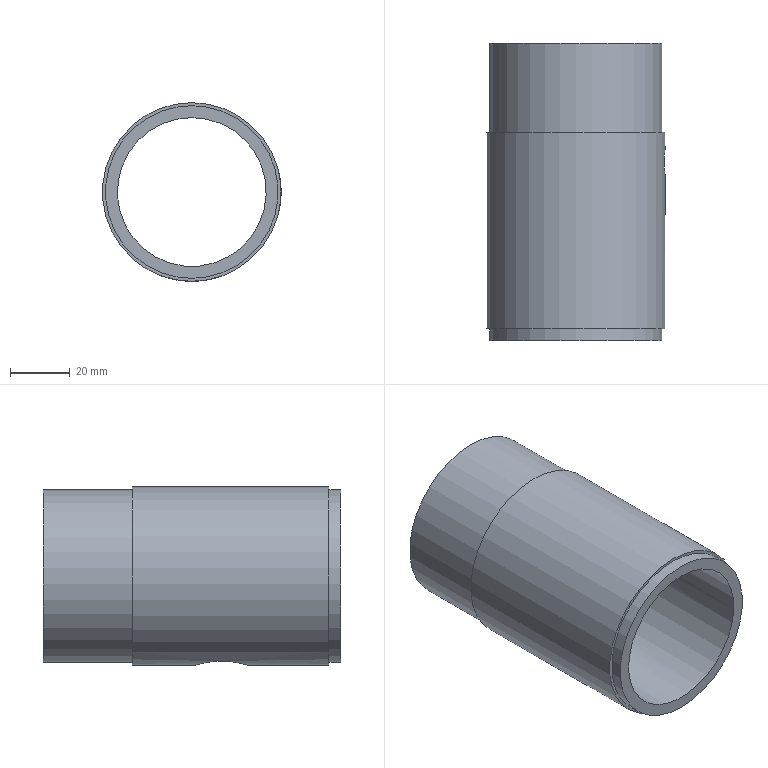Part | STEP file | JBJ-P-1008-02 | 1 solid | 10 faces | box 60 x 100 x 60 mm | volume 77175 mm3 | cylinder 6 | plane 3 | cone 1 | commonest cylinder face diameters 58 x2 8.8 x1 18 x1 50 x1 60 x1
STEP:
#1=CARTESIAN_POINT('',(0.,49.,-30.));
#2=VERTEX_POINT('',#1);
#3=CARTESIAN_POINT('',(0.,49.,-30.));
#4=CARTESIAN_POINT('',(-0.5983,49.,-30.));
#5=CARTESIAN_POINT('',(-1.186,48.941,-29.982));
#6=CARTESIAN_POINT('',(-2.052,48.768,-29.931));
#7=CARTESIAN_POINT('',(-2.338,48.696,-29.91));
#8=CARTESIAN_POINT('',(-2.906,48.523,-29.86));
#9=CARTESIAN_POINT('',(-3.187,48.422,-29.832));
#10=CARTESIAN_POINT('',(-4.003,48.082,-29.737));
#11=CARTESIAN_POINT('',(-4.518,47.806,-29.662));
#12=CARTESIAN_POINT('',(-5.25,47.316,-29.538));
#13=CARTESIAN_POINT('',(-5.488,47.139,-29.495));
#14=CARTESIAN_POINT('',(-5.943,46.765,-29.406));
#15=CARTESIAN_POINT('',(-6.16,46.569,-29.362));
#16=CARTESIAN_POINT('',(-6.778,45.95,-29.227));
#17=CARTESIAN_POINT('',(-7.149,45.499,-29.138));
#18=CARTESIAN_POINT('',(-7.807,44.516,-28.968));
#19=CARTESIAN_POINT('',(-8.084,43.998,-28.891));
#20=CARTESIAN_POINT('',(-8.422,43.187,-28.794));
#21=CARTESIAN_POINT('',(-8.521,42.911,-28.764));
#22=CARTESIAN_POINT('',(-8.694,42.346,-28.713));
#23=CARTESIAN_POINT('',(-8.767,42.056,-28.69));
#24=CARTESIAN_POINT('',(-8.942,41.183,-28.637));
#25=CARTESIAN_POINT('',(-9.,40.597,-28.618));
#26=CARTESIAN_POINT('',(-9.,39.415,-28.618));
#27=CARTESIAN_POINT('',(-8.941,38.815,-28.637));
#28=CARTESIAN_POINT('',(-8.71,37.658,-28.708));
#29=CARTESIAN_POINT('',(-8.539,37.095,-28.76));
#30=CARTESIAN_POINT('',(-8.198,36.275,-28.858));
#31=CARTESIAN_POINT('',(-8.071,36.006,-28.894));
#32=CARTESIAN_POINT('',(-7.793,35.488,-28.971));
#33=CARTESIAN_POINT('',(-7.642,35.238,-29.011));
#34=CARTESIAN_POINT('',(-7.317,34.752,-29.094));
#35=CARTESIAN_POINT('',(-7.143,34.517,-29.138));
#36=CARTESIAN_POINT('',(-6.771,34.063,-29.227));
#37=CARTESIAN_POINT('',(-6.572,33.844,-29.272));
#38=CARTESIAN_POINT('',(-5.949,33.221,-29.407));
#39=CARTESIAN_POINT('',(-5.498,32.851,-29.496));
#40=CARTESIAN_POINT('',(-4.526,32.199,-29.661));
#41=CARTESIAN_POINT('',(-3.999,31.916,-29.737));
#42=CARTESIAN_POINT('',(-2.914,31.465,-29.863));
#43=CARTESIAN_POINT('',(-2.353,31.293,-29.913));
#44=CARTESIAN_POINT('',(-1.481,31.118,-29.965));
#45=CARTESIAN_POINT('',(-1.184,31.073,-29.978));
#46=CARTESIAN_POINT('',(-0.5936,31.015,-29.996));
#47=CARTESIAN_POINT('',(-0.003551,30.986,-30.004));
#48=CARTESIAN_POINT('',(0.5855,31.014,-29.996));
#49=CARTESIAN_POINT('',(1.174,31.072,-29.978));
#50=CARTESIAN_POINT('',(1.469,31.116,-29.965));
#51=CARTESIAN_POINT('',(2.346,31.291,-29.914));
#52=CARTESIAN_POINT('',(2.909,31.463,-29.864));
#53=CARTESIAN_POINT('',(3.994,31.913,-29.738));
#54=CARTESIAN_POINT('',(4.521,32.196,-29.662));
#55=CARTESIAN_POINT('',(5.495,32.848,-29.497));
#56=CARTESIAN_POINT('',(5.946,33.218,-29.408));
#57=CARTESIAN_POINT('',(6.569,33.841,-29.273));
#58=CARTESIAN_POINT('',(6.768,34.061,-29.227));
#59=CARTESIAN_POINT('',(7.141,34.514,-29.138));
#60=CARTESIAN_POINT('',(7.315,34.749,-29.095));
#61=CARTESIAN_POINT('',(7.802,35.476,-28.97));
#62=CARTESIAN_POINT('',(8.081,35.993,-28.892));
#63=CARTESIAN_POINT('',(8.537,37.09,-28.761));
#64=CARTESIAN_POINT('',(8.708,37.653,-28.709));
#65=CARTESIAN_POINT('',(8.882,38.518,-28.655));
#66=CARTESIAN_POINT('',(8.926,38.81,-28.641));
#67=CARTESIAN_POINT('',(8.985,39.401,-28.623));
#68=CARTESIAN_POINT('',(9.,39.701,-28.618));
#69=CARTESIAN_POINT('',(9.,40.591,-28.618));
#70=CARTESIAN_POINT('',(8.942,41.177,-28.637));
#71=CARTESIAN_POINT('',(8.769,42.047,-28.69));
#72=CARTESIAN_POINT('',(8.696,42.337,-28.712));
#73=CARTESIAN_POINT('',(8.524,42.905,-28.764));
#74=CARTESIAN_POINT('',(8.424,43.182,-28.793));
#75=CARTESIAN_POINT('',(8.086,43.995,-28.891));
#76=CARTESIAN_POINT('',(7.809,44.513,-28.968));
#77=CARTESIAN_POINT('',(7.151,45.497,-29.137));
#78=CARTESIAN_POINT('',(6.78,45.948,-29.227));
#79=CARTESIAN_POINT('',(6.161,46.567,-29.361));
#80=CARTESIAN_POINT('',(5.944,46.764,-29.406));
#81=CARTESIAN_POINT('',(5.49,47.137,-29.494));
#82=CARTESIAN_POINT('',(5.252,47.315,-29.538));
#83=CARTESIAN_POINT('',(4.52,47.805,-29.662));
#84=CARTESIAN_POINT('',(4.005,48.081,-29.736));
#85=CARTESIAN_POINT('',(2.919,48.534,-29.863));
#86=CARTESIAN_POINT('',(2.345,48.709,-29.914));
#87=CARTESIAN_POINT('',(1.187,48.941,-29.982));
#88=CARTESIAN_POINT('',(0.5983,49.,-30.));
#89=CARTESIAN_POINT('',(0.,49.,-30.));
#90=B_SPLINE_CURVE_WITH_KNOTS('',3,(#3,#4,#5,#6,#7,#8,#9,#10,#11,#12,#13,#14,#15,#16,#17,#18,#19,#20,#21,#22,#23,#24,#25,#26,#27,#28,#29,#30,#31,#32,#33,#34,#35,#36,#37,#38,#39,#40,#41,#42,#43,#44,#45,#46,#47,#48,#49,#50,#51,#52,#53,#54,#55,#56,#57,#58,#59,#60,#61,#62,#63,#64,#65,#66,#67,#68,#69,#70,#71,#72,#73,#74,#75,#76,#77,#78,#79,#80,#81,#82,#83,#84,#85,#86,#87,#88,#89),.UNSPECIFIED.,.T.,.F.,(4,2,2,2,2,2,2,2,2,2,2,2,2,2,2,2,2,2,2,2,2,2,1,2,2,2,2,2,2,2,2,2,2,2,2,2,2,2,2,2,2,2,2,4),(0.,0.001769,0.002653,0.003537,0.005306,0.00619,0.007075,0.008843,0.01061,0.0115,0.01238,0.01415,0.01592,0.01769,0.01857,0.01946,0.02034,0.02122,0.02299,0.02476,0.02653,0.02741,0.0283,0.02918,0.03007,0.03184,0.0336,0.03537,0.03626,0.03714,0.03891,0.04068,0.04156,0.04245,0.04422,0.0451,0.04598,0.04775,0.04952,0.05041,0.05129,0.05306,0.05483,0.0566),.UNSPECIFIED.);
#91=EDGE_CURVE('',#2,#2,#90,.T.);
#92=ORIENTED_EDGE('',*,*,#91,.T.);
#93=EDGE_LOOP('',(#92));
#94=FACE_BOUND('',#93,.T.);
#95=CARTESIAN_POINT('',(30.,55.6,0.));
#96=VERTEX_POINT('',#95);
#97=CARTESIAN_POINT('',(30.,55.6,0.));
#98=CARTESIAN_POINT('',(30.,55.6,0.2911));
#99=CARTESIAN_POINT('',(29.996,55.629,0.5773));
#100=CARTESIAN_POINT('',(29.98,55.741,1.14));
#101=CARTESIAN_POINT('',(29.968,55.825,1.42));
#102=CARTESIAN_POINT('',(29.938,56.046,1.952));
#103=CARTESIAN_POINT('',(29.92,56.182,2.205));
#104=CARTESIAN_POINT('',(29.881,56.501,2.683));
#105=CARTESIAN_POINT('',(29.859,56.686,2.909));
#106=CARTESIAN_POINT('',(29.817,57.092,3.314));
#107=CARTESIAN_POINT('',(29.796,57.313,3.496));
#108=CARTESIAN_POINT('',(29.757,57.794,3.818));
#109=CARTESIAN_POINT('',(29.738,58.049,3.954));
#110=CARTESIAN_POINT('',(29.708,58.579,4.174));
#111=CARTESIAN_POINT('',(29.696,58.856,4.259));
#112=CARTESIAN_POINT('',(29.68,59.424,4.372));
#113=CARTESIAN_POINT('',(29.676,59.71,4.4));
#114=CARTESIAN_POINT('',(29.676,60.285,4.4));
#115=CARTESIAN_POINT('',(29.68,60.577,4.372));
#116=CARTESIAN_POINT('',(29.696,61.141,4.259));
#117=CARTESIAN_POINT('',(29.708,61.416,4.176));
#118=CARTESIAN_POINT('',(29.738,61.949,3.955));
#119=CARTESIAN_POINT('',(29.757,62.206,3.818));
#120=CARTESIAN_POINT('',(29.796,62.683,3.499));
#121=CARTESIAN_POINT('',(29.817,62.905,3.317));
#122=CARTESIAN_POINT('',(29.859,63.315,2.907));
#123=CARTESIAN_POINT('',(29.881,63.497,2.686));
#124=CARTESIAN_POINT('',(29.919,63.816,2.21));
#125=CARTESIAN_POINT('',(29.938,63.954,1.952));
#126=CARTESIAN_POINT('',(29.968,64.175,1.42));
#127=CARTESIAN_POINT('',(29.979,64.258,1.145));
#128=CARTESIAN_POINT('',(29.996,64.371,0.5809));
#129=CARTESIAN_POINT('',(30.,64.4,0.289));
#130=CARTESIAN_POINT('',(30.,64.4,-0.2857));
#131=CARTESIAN_POINT('',(29.996,64.372,-0.5715));
#132=CARTESIAN_POINT('',(29.98,64.26,-1.14));
#133=CARTESIAN_POINT('',(29.968,64.175,-1.418));
#134=CARTESIAN_POINT('',(29.938,63.956,-1.947));
#135=CARTESIAN_POINT('',(29.92,63.819,-2.204));
#136=CARTESIAN_POINT('',(29.881,63.499,-2.684));
#137=CARTESIAN_POINT('',(29.86,63.317,-2.905));
#138=CARTESIAN_POINT('',(29.817,62.912,-3.311));
#139=CARTESIAN_POINT('',(29.796,62.686,-3.497));
#140=CARTESIAN_POINT('',(29.757,62.208,-3.816));
#141=CARTESIAN_POINT('',(29.739,61.956,-3.952));
#142=CARTESIAN_POINT('',(29.708,61.423,-4.173));
#143=CARTESIAN_POINT('',(29.696,61.144,-4.258));
#144=CARTESIAN_POINT('',(29.68,60.581,-4.371));
#145=CARTESIAN_POINT('',(29.676,60.295,-4.4));
#146=CARTESIAN_POINT('',(29.676,59.713,-4.4));
#147=CARTESIAN_POINT('',(29.68,59.427,-4.372));
#148=CARTESIAN_POINT('',(29.696,58.864,-4.26));
#149=CARTESIAN_POINT('',(29.708,58.584,-4.176));
#150=CARTESIAN_POINT('',(29.738,58.051,-3.955));
#151=CARTESIAN_POINT('',(29.756,57.798,-3.82));
#152=CARTESIAN_POINT('',(29.795,57.32,-3.501));
#153=CARTESIAN_POINT('',(29.817,57.094,-3.316));
#154=CARTESIAN_POINT('',(29.859,56.688,-2.911));
#155=CARTESIAN_POINT('',(29.88,56.506,-2.69));
#156=CARTESIAN_POINT('',(29.92,56.184,-2.209));
#157=CARTESIAN_POINT('',(29.937,56.047,-1.954));
#158=CARTESIAN_POINT('',(29.967,55.827,-1.425));
#159=CARTESIAN_POINT('',(29.979,55.742,-1.147));
#160=CARTESIAN_POINT('',(29.996,55.629,-0.5788));
#161=CARTESIAN_POINT('',(30.,55.6,-0.2911));
#162=CARTESIAN_POINT('',(30.,55.6,0.));
#163=B_SPLINE_CURVE_WITH_KNOTS('',3,(#97,#98,#99,#100,#101,#102,#103,#104,#105,#106,#107,#108,#109,#110,#111,#112,#113,#114,#115,#116,#117,#118,#119,#120,#121,#122,#123,#124,#125,#126,#127,#128,#129,#130,#131,#132,#133,#134,#135,#136,#137,#138,#139,#140,#141,#142,#143,#144,#145,#146,#147,#148,#149,#150,#151,#152,#153,#154,#155,#156,#157,#158,#159,#160,#161,#162),.UNSPECIFIED.,.T.,.F.,(4,2,2,2,2,2,2,2,2,2,2,2,2,2,2,2,2,2,2,2,2,2,2,2,2,2,2,2,2,2,2,2,4),(0.,0.0008608,0.001722,0.002582,0.003443,0.004304,0.005165,0.006026,0.006887,0.007747,0.008608,0.009469,0.01033,0.01119,0.01205,0.01291,0.01377,0.01463,0.01549,0.01636,0.01722,0.01808,0.01894,0.0198,0.02066,0.02152,0.02238,0.02324,0.0241,0.02496,0.02582,0.02669,0.02755),.UNSPECIFIED.);
#164=EDGE_CURVE('',#96,#96,#163,.T.);
#165=ORIENTED_EDGE('',*,*,#164,.T.);
#166=EDGE_LOOP('',(#165));
#167=FACE_BOUND('',#166,.T.);
#168=CARTESIAN_POINT('',(0.,4.,-30.));
#169=VERTEX_POINT('',#168);
#170=CARTESIAN_POINT('',(0.,4.,0.));
#171=DIRECTION('',(0.,-1.,0.));
#172=DIRECTION('',(0.,0.,-1.));
#173=AXIS2_PLACEMENT_3D('',#170,#171,#172);
#174=CIRCLE('',#173,30.);
#175=EDGE_CURVE('',#169,#169,#174,.T.);
#176=ORIENTED_EDGE('',*,*,#175,.F.);
#177=EDGE_LOOP('',(#176));
#178=FACE_OUTER_BOUND('',#177,.T.);
#179=CARTESIAN_POINT('',(0.,70.,30.));
#180=VERTEX_POINT('',#179);
#181=CARTESIAN_POINT('',(0.,70.,0.));
#182=DIRECTION('',(0.,1.,0.));
#183=DIRECTION('',(0.,0.,1.));
#184=AXIS2_PLACEMENT_3D('',#181,#182,#183);
#185=CIRCLE('',#184,30.);
#186=EDGE_CURVE('',#180,#180,#185,.T.);
#187=ORIENTED_EDGE('',*,*,#186,.F.);
#188=EDGE_LOOP('',(#187));
#189=FACE_OUTER_BOUND('',#188,.T.);
#190=CARTESIAN_POINT('',(0.,100.,0.));
#191=DIRECTION('',(0.,-1.,0.));
#192=DIRECTION('',(0.,0.,-1.));
#193=AXIS2_PLACEMENT_3D('',#190,#191,#192);
#194=CYLINDRICAL_SURFACE('',#193,30.);
#195=ADVANCED_FACE('',(#94,#167,#178,#189),#194,.T.);
#196=CARTESIAN_POINT('',(0.,0.,25.));
#197=VERTEX_POINT('',#196);
#198=CARTESIAN_POINT('',(0.,0.,0.));
#199=DIRECTION('',(0.,1.,0.));
#200=DIRECTION('',(0.,0.,1.));
#201=AXIS2_PLACEMENT_3D('',#198,#199,#200);
#202=CIRCLE('',#201,25.);
#203=EDGE_CURVE('',#197,#197,#202,.T.);
#204=ORIENTED_EDGE('',*,*,#203,.T.);
#205=EDGE_LOOP('',(#204));
#206=FACE_BOUND('',#205,.T.);
#207=CARTESIAN_POINT('',(0.,0.,-29.));
#208=VERTEX_POINT('',#207);
#209=CARTESIAN_POINT('',(0.,0.,0.));
#210=DIRECTION('',(0.,-1.,0.));
#211=DIRECTION('',(0.,0.,-1.));
#212=AXIS2_PLACEMENT_3D('',#209,#210,#211);
#213=CIRCLE('',#212,29.);
#214=EDGE_CURVE('',#208,#208,#213,.T.);
#215=ORIENTED_EDGE('',*,*,#214,.T.);
#216=EDGE_LOOP('',(#215));
#217=FACE_OUTER_BOUND('',#216,.T.);
#218=CARTESIAN_POINT('',(0.,0.,0.));
#219=DIRECTION('',(0.,1.,0.));
#220=DIRECTION('',(0.,0.,1.));
#221=AXIS2_PLACEMENT_3D('',#218,#219,#220);
#222=PLANE('',#221);
#223=ADVANCED_FACE('',(#206,#217),#222,.F.);
#224=CARTESIAN_POINT('',(0.,96.,25.));
#225=VERTEX_POINT('',#224);
#226=CARTESIAN_POINT('',(0.,96.,0.));
#227=DIRECTION('',(0.,1.,0.));
#228=DIRECTION('',(0.,0.,1.));
#229=AXIS2_PLACEMENT_3D('',#226,#227,#228);
#230=CIRCLE('',#229,25.);
#231=EDGE_CURVE('',#225,#225,#230,.T.);
#232=ORIENTED_EDGE('',*,*,#231,.T.);
#233=EDGE_LOOP('',(#232));
#234=FACE_OUTER_BOUND('',#233,.T.);
#235=CARTESIAN_POINT('',(0.,49.,-25.));
#236=VERTEX_POINT('',#235);
#237=CARTESIAN_POINT('',(0.,49.,-25.));
#238=CARTESIAN_POINT('',(-0.6,49.,-25.));
#239=CARTESIAN_POINT('',(-1.189,48.941,-24.978));
#240=CARTESIAN_POINT('',(-2.057,48.767,-24.917));
#241=CARTESIAN_POINT('',(-2.344,48.695,-24.892));
#242=CARTESIAN_POINT('',(-2.912,48.521,-24.831));
#243=CARTESIAN_POINT('',(-3.193,48.42,-24.797));
#244=CARTESIAN_POINT('',(-4.009,48.079,-24.683));
#245=CARTESIAN_POINT('',(-4.524,47.803,-24.592));
#246=CARTESIAN_POINT('',(-5.255,47.313,-24.443));
#247=CARTESIAN_POINT('',(-5.492,47.136,-24.39));
#248=CARTESIAN_POINT('',(-5.945,46.763,-24.284));
#249=CARTESIAN_POINT('',(-6.161,46.567,-24.23));
#250=CARTESIAN_POINT('',(-6.778,45.95,-24.067));
#251=CARTESIAN_POINT('',(-7.149,45.499,-23.959));
#252=CARTESIAN_POINT('',(-7.806,44.518,-23.753));
#253=CARTESIAN_POINT('',(-8.082,44.003,-23.659));
#254=CARTESIAN_POINT('',(-8.42,43.193,-23.54));
#255=CARTESIAN_POINT('',(-8.52,42.916,-23.504));
#256=CARTESIAN_POINT('',(-8.693,42.35,-23.44));
#257=CARTESIAN_POINT('',(-8.766,42.059,-23.413));
#258=CARTESIAN_POINT('',(-8.941,41.186,-23.347));
#259=CARTESIAN_POINT('',(-9.,40.599,-23.324));
#260=CARTESIAN_POINT('',(-9.,39.71,-23.324));
#261=CARTESIAN_POINT('',(-8.986,39.411,-23.329));
#262=CARTESIAN_POINT('',(-8.927,38.816,-23.352));
#263=CARTESIAN_POINT('',(-8.883,38.522,-23.369));
#264=CARTESIAN_POINT('',(-8.709,37.653,-23.434));
#265=CARTESIAN_POINT('',(-8.537,37.089,-23.498));
#266=CARTESIAN_POINT('',(-8.081,35.993,-23.659));
#267=CARTESIAN_POINT('',(-7.802,35.476,-23.754));
#268=CARTESIAN_POINT('',(-7.315,34.749,-23.906));
#269=CARTESIAN_POINT('',(-7.141,34.514,-23.959));
#270=CARTESIAN_POINT('',(-6.768,34.061,-24.067));
#271=CARTESIAN_POINT('',(-6.57,33.842,-24.122));
#272=CARTESIAN_POINT('',(-5.95,33.222,-24.285));
#273=CARTESIAN_POINT('',(-5.501,32.853,-24.392));
#274=CARTESIAN_POINT('',(-4.772,32.363,-24.542));
#275=CARTESIAN_POINT('',(-4.518,32.211,-24.59));
#276=CARTESIAN_POINT('',(-3.997,31.931,-24.68));
#277=CARTESIAN_POINT('',(-3.732,31.805,-24.721));
#278=CARTESIAN_POINT('',(-2.92,31.467,-24.835));
#279=CARTESIAN_POINT('',(-2.358,31.294,-24.895));
#280=CARTESIAN_POINT('',(-1.482,31.118,-24.958));
#281=CARTESIAN_POINT('',(-1.185,31.073,-24.974));
#282=CARTESIAN_POINT('',(-0.5942,31.015,-24.995));
#283=CARTESIAN_POINT('',(-0.003306,30.985,-25.005));
#284=CARTESIAN_POINT('',(0.5878,31.014,-24.995));
#285=CARTESIAN_POINT('',(1.179,31.073,-24.974));
#286=CARTESIAN_POINT('',(1.476,31.117,-24.958));
#287=CARTESIAN_POINT('',(2.352,31.292,-24.896));
#288=CARTESIAN_POINT('',(2.915,31.465,-24.836));
#289=CARTESIAN_POINT('',(3.731,31.804,-24.722));
#290=CARTESIAN_POINT('',(3.999,31.932,-24.68));
#291=CARTESIAN_POINT('',(4.52,32.212,-24.589));
#292=CARTESIAN_POINT('',(4.771,32.363,-24.542));
#293=CARTESIAN_POINT('',(5.499,32.851,-24.393));
#294=CARTESIAN_POINT('',(5.95,33.221,-24.286));
#295=CARTESIAN_POINT('',(6.781,34.054,-24.067));
#296=CARTESIAN_POINT('',(7.153,34.506,-23.957));
#297=CARTESIAN_POINT('',(7.639,35.232,-23.805));
#298=CARTESIAN_POINT('',(7.79,35.482,-23.756));
#299=CARTESIAN_POINT('',(8.068,36.,-23.663));
#300=CARTESIAN_POINT('',(8.195,36.269,-23.619));
#301=CARTESIAN_POINT('',(8.536,37.087,-23.499));
#302=CARTESIAN_POINT('',(8.708,37.649,-23.435));
#303=CARTESIAN_POINT('',(8.882,38.517,-23.369));
#304=CARTESIAN_POINT('',(8.926,38.81,-23.352));
#305=CARTESIAN_POINT('',(8.985,39.406,-23.329));
#306=CARTESIAN_POINT('',(9.,39.705,-23.324));
#307=CARTESIAN_POINT('',(9.,40.594,-23.324));
#308=CARTESIAN_POINT('',(8.942,41.182,-23.347));
#309=CARTESIAN_POINT('',(8.767,42.057,-23.413));
#310=CARTESIAN_POINT('',(8.693,42.348,-23.44));
#311=CARTESIAN_POINT('',(8.52,42.914,-23.503));
#312=CARTESIAN_POINT('',(8.42,43.191,-23.54));
#313=CARTESIAN_POINT('',(8.195,43.733,-23.619));
#314=CARTESIAN_POINT('',(8.069,43.998,-23.663));
#315=CARTESIAN_POINT('',(7.791,44.516,-23.756));
#316=CARTESIAN_POINT('',(7.638,44.77,-23.805));
#317=CARTESIAN_POINT('',(7.147,45.502,-23.959));
#318=CARTESIAN_POINT('',(6.777,45.951,-24.068));
#319=CARTESIAN_POINT('',(5.951,46.777,-24.285));
#320=CARTESIAN_POINT('',(5.492,47.154,-24.394));
#321=CARTESIAN_POINT('',(4.521,47.804,-24.593));
#322=CARTESIAN_POINT('',(4.007,48.08,-24.683));
#323=CARTESIAN_POINT('',(3.189,48.421,-24.797));
#324=CARTESIAN_POINT('',(2.907,48.523,-24.832));
#325=CARTESIAN_POINT('',(2.341,48.695,-24.892));
#326=CARTESIAN_POINT('',(2.055,48.767,-24.917));
#327=CARTESIAN_POINT('',(1.189,48.941,-24.978));
#328=CARTESIAN_POINT('',(0.6,49.,-25.));
#329=CARTESIAN_POINT('',(0.,49.,-25.));
#330=B_SPLINE_CURVE_WITH_KNOTS('',3,(#237,#238,#239,#240,#241,#242,#243,#244,#245,#246,#247,#248,#249,#250,#251,#252,#253,#254,#255,#256,#257,#258,#259,#260,#261,#262,#263,#264,#265,#266,#267,#268,#269,#270,#271,#272,#273,#274,#275,#276,#277,#278,#279,#280,#281,#282,#283,#284,#285,#286,#287,#288,#289,#290,#291,#292,#293,#294,#295,#296,#297,#298,#299,#300,#301,#302,#303,#304,#305,#306,#307,#308,#309,#310,#311,#312,#313,#314,#315,#316,#317,#318,#319,#320,#321,#322,#323,#324,#325,#326,#327,#328,#329),.UNSPECIFIED.,.T.,.F.,(4,2,2,2,2,2,2,2,2,2,2,2,2,2,2,2,2,2,2,2,2,2,2,1,2,2,2,2,2,2,2,2,2,2,2,2,2,2,2,2,2,2,2,2,2,2,4),(0.,0.001773,0.00266,0.003547,0.00532,0.006207,0.007094,0.008867,0.01064,0.01153,0.01241,0.01419,0.01507,0.01596,0.01773,0.01951,0.02039,0.02128,0.02305,0.02394,0.02483,0.0266,0.02749,0.02838,0.02926,0.03015,0.03192,0.03281,0.0337,0.03547,0.03724,0.03813,0.03902,0.04079,0.04168,0.04256,0.04434,0.04522,0.04611,0.047,0.04788,0.04966,0.05143,0.0532,0.05409,0.05498,0.05675),.UNSPECIFIED.);
#331=EDGE_CURVE('',#236,#236,#330,.T.);
#332=ORIENTED_EDGE('',*,*,#331,.F.);
#333=EDGE_LOOP('',(#332));
#334=FACE_BOUND('',#333,.T.);
#335=CARTESIAN_POINT('',(24.61,60.,4.4));
#336=VERTEX_POINT('',#335);
#337=CARTESIAN_POINT('',(24.61,60.,4.4));
#338=CARTESIAN_POINT('',(24.61,60.291,4.4));
#339=CARTESIAN_POINT('',(24.615,60.578,4.371));
#340=CARTESIAN_POINT('',(24.635,61.141,4.259));
#341=CARTESIAN_POINT('',(24.649,61.42,4.174));
#342=CARTESIAN_POINT('',(24.686,61.953,3.953));
#343=CARTESIAN_POINT('',(24.707,62.205,3.818));
#344=CARTESIAN_POINT('',(24.754,62.683,3.499));
#345=CARTESIAN_POINT('',(24.78,62.909,3.313));
#346=CARTESIAN_POINT('',(24.831,63.314,2.908));
#347=CARTESIAN_POINT('',(24.856,63.496,2.687));
#348=CARTESIAN_POINT('',(24.904,63.818,2.206));
#349=CARTESIAN_POINT('',(24.925,63.954,1.951));
#350=CARTESIAN_POINT('',(24.961,64.174,1.422));
#351=CARTESIAN_POINT('',(24.975,64.258,1.144));
#352=CARTESIAN_POINT('',(24.995,64.372,0.576));
#353=CARTESIAN_POINT('',(25.,64.4,0.2901));
#354=CARTESIAN_POINT('',(25.,64.4,-0.285));
#355=CARTESIAN_POINT('',(24.995,64.371,-0.5772));
#356=CARTESIAN_POINT('',(24.976,64.259,-1.142));
#357=CARTESIAN_POINT('',(24.961,64.176,-1.416));
#358=CARTESIAN_POINT('',(24.925,63.955,-1.95));
#359=CARTESIAN_POINT('',(24.904,63.817,-2.207));
#360=CARTESIAN_POINT('',(24.857,63.499,-2.683));
#361=CARTESIAN_POINT('',(24.831,63.317,-2.906));
#362=CARTESIAN_POINT('',(24.78,62.907,-3.315));
#363=CARTESIAN_POINT('',(24.755,62.686,-3.497));
#364=CARTESIAN_POINT('',(24.708,62.21,-3.816));
#365=CARTESIAN_POINT('',(24.686,61.952,-3.954));
#366=CARTESIAN_POINT('',(24.649,61.42,-4.174));
#367=CARTESIAN_POINT('',(24.635,61.146,-4.258));
#368=CARTESIAN_POINT('',(24.615,60.581,-4.371));
#369=CARTESIAN_POINT('',(24.61,60.289,-4.4));
#370=CARTESIAN_POINT('',(24.61,59.714,-4.4));
#371=CARTESIAN_POINT('',(24.615,59.428,-4.372));
#372=CARTESIAN_POINT('',(24.635,58.859,-4.259));
#373=CARTESIAN_POINT('',(24.649,58.582,-4.175));
#374=CARTESIAN_POINT('',(24.685,58.052,-3.956));
#375=CARTESIAN_POINT('',(24.707,57.795,-3.819));
#376=CARTESIAN_POINT('',(24.755,57.316,-3.498));
#377=CARTESIAN_POINT('',(24.78,57.095,-3.317));
#378=CARTESIAN_POINT('',(24.831,56.689,-2.912));
#379=CARTESIAN_POINT('',(24.856,56.503,-2.686));
#380=CARTESIAN_POINT('',(24.903,56.184,-2.209));
#381=CARTESIAN_POINT('',(24.925,56.048,-1.957));
#382=CARTESIAN_POINT('',(24.961,55.827,-1.423));
#383=CARTESIAN_POINT('',(24.975,55.742,-1.144));
#384=CARTESIAN_POINT('',(24.995,55.629,-0.5818));
#385=CARTESIAN_POINT('',(25.,55.6,-0.2941));
#386=CARTESIAN_POINT('',(25.,55.6,0.2873));
#387=CARTESIAN_POINT('',(24.995,55.628,0.5734));
#388=CARTESIAN_POINT('',(24.976,55.74,1.137));
#389=CARTESIAN_POINT('',(24.961,55.825,1.417));
#390=CARTESIAN_POINT('',(24.925,56.045,1.949));
#391=CARTESIAN_POINT('',(24.904,56.18,2.202));
#392=CARTESIAN_POINT('',(24.857,56.499,2.681));
#393=CARTESIAN_POINT('',(24.831,56.684,2.906));
#394=CARTESIAN_POINT('',(24.781,57.089,3.311));
#395=CARTESIAN_POINT('',(24.755,57.31,3.494));
#396=CARTESIAN_POINT('',(24.707,57.791,3.817));
#397=CARTESIAN_POINT('',(24.686,58.045,3.952));
#398=CARTESIAN_POINT('',(24.65,58.574,4.172));
#399=CARTESIAN_POINT('',(24.635,58.853,4.258));
#400=CARTESIAN_POINT('',(24.615,59.421,4.371));
#401=CARTESIAN_POINT('',(24.61,59.709,4.4));
#402=CARTESIAN_POINT('',(24.61,60.,4.4));
#403=B_SPLINE_CURVE_WITH_KNOTS('',3,(#337,#338,#339,#340,#341,#342,#343,#344,#345,#346,#347,#348,#349,#350,#351,#352,#353,#354,#355,#356,#357,#358,#359,#360,#361,#362,#363,#364,#365,#366,#367,#368,#369,#370,#371,#372,#373,#374,#375,#376,#377,#378,#379,#380,#381,#382,#383,#384,#385,#386,#387,#388,#389,#390,#391,#392,#393,#394,#395,#396,#397,#398,#399,#400,#401,#402),.UNSPECIFIED.,.T.,.F.,(4,2,2,2,2,2,2,2,2,2,2,2,2,2,2,2,2,2,2,2,2,2,2,2,2,2,2,2,2,2,2,2,4),(0.,0.0008613,0.001723,0.002584,0.003445,0.004307,0.005168,0.006029,0.006891,0.007752,0.008613,0.009475,0.01034,0.0112,0.01206,0.01292,0.01378,0.01464,0.0155,0.01637,0.01723,0.01809,0.01895,0.01981,0.02067,0.02153,0.02239,0.02326,0.02412,0.02498,0.02584,0.0267,0.02756),.UNSPECIFIED.);
#404=EDGE_CURVE('',#336,#336,#403,.T.);
#405=ORIENTED_EDGE('',*,*,#404,.F.);
#406=EDGE_LOOP('',(#405));
#407=FACE_BOUND('',#406,.T.);
#408=ORIENTED_EDGE('',*,*,#203,.F.);
#409=EDGE_LOOP('',(#408));
#410=FACE_OUTER_BOUND('',#409,.T.);
#411=CARTESIAN_POINT('',(0.,100.,0.));
#412=DIRECTION('',(0.,-1.,0.));
#413=DIRECTION('',(0.,0.,-1.));
#414=AXIS2_PLACEMENT_3D('',#411,#412,#413);
#415=CYLINDRICAL_SURFACE('',#414,25.);
#416=ADVANCED_FACE('',(#234,#334,#407,#410),#415,.F.);
#417=CARTESIAN_POINT('',(0.,4.,-29.));
#418=VERTEX_POINT('',#417);
#419=CARTESIAN_POINT('',(0.,4.,0.));
#420=DIRECTION('',(0.,-1.,0.));
#421=DIRECTION('',(0.,0.,-1.));
#422=AXIS2_PLACEMENT_3D('',#419,#420,#421);
#423=CIRCLE('',#422,29.);
#424=EDGE_CURVE('',#418,#418,#423,.T.);
#425=ORIENTED_EDGE('',*,*,#424,.F.);
#426=EDGE_LOOP('',(#425));
#427=FACE_BOUND('',#426,.T.);
#428=ORIENTED_EDGE('',*,*,#175,.T.);
#429=EDGE_LOOP('',(#428));
#430=FACE_OUTER_BOUND('',#429,.T.);
#431=CARTESIAN_POINT('',(0.,4.,0.));
#432=DIRECTION('',(0.,-1.,0.));
#433=DIRECTION('',(0.,0.,-1.));
#434=AXIS2_PLACEMENT_3D('',#431,#432,#433);
#435=PLANE('',#434);
#436=ADVANCED_FACE('',(#427,#430),#435,.T.);
#437=ORIENTED_EDGE('',*,*,#424,.T.);
#438=EDGE_LOOP('',(#437));
#439=FACE_OUTER_BOUND('',#438,.T.);
#440=ORIENTED_EDGE('',*,*,#214,.F.);
#441=EDGE_LOOP('',(#440));
#442=FACE_OUTER_BOUND('',#441,.T.);
#443=CARTESIAN_POINT('',(0.,4.,0.));
#444=DIRECTION('',(0.,-1.,0.));
#445=DIRECTION('',(0.,0.,-1.));
#446=AXIS2_PLACEMENT_3D('',#443,#444,#445);
#447=CYLINDRICAL_SURFACE('',#446,29.);
#448=ADVANCED_FACE('',(#439,#442),#447,.T.);
#449=CARTESIAN_POINT('',(0.,70.,29.));
#450=VERTEX_POINT('',#449);
#451=CARTESIAN_POINT('',(0.,70.,0.));
#452=DIRECTION('',(0.,1.,0.));
#453=DIRECTION('',(0.,0.,1.));
#454=AXIS2_PLACEMENT_3D('',#451,#452,#453);
#455=CIRCLE('',#454,29.);
#456=EDGE_CURVE('',#450,#450,#455,.T.);
#457=ORIENTED_EDGE('',*,*,#456,.F.);
#458=EDGE_LOOP('',(#457));
#459=FACE_BOUND('',#458,.T.);
#460=ORIENTED_EDGE('',*,*,#186,.T.);
#461=EDGE_LOOP('',(#460));
#462=FACE_OUTER_BOUND('',#461,.T.);
#463=CARTESIAN_POINT('',(0.,70.,0.));
#464=DIRECTION('',(0.,1.,0.));
#465=DIRECTION('',(0.,0.,1.));
#466=AXIS2_PLACEMENT_3D('',#463,#464,#465);
#467=PLANE('',#466);
#468=ADVANCED_FACE('',(#459,#462),#467,.T.);
#469=ORIENTED_EDGE('',*,*,#456,.T.);
#470=EDGE_LOOP('',(#469));
#471=FACE_OUTER_BOUND('',#470,.T.);
#472=CARTESIAN_POINT('',(0.,100.,29.));
#473=VERTEX_POINT('',#472);
#474=CARTESIAN_POINT('',(0.,100.,0.));
#475=DIRECTION('',(0.,1.,0.));
#476=DIRECTION('',(0.,0.,1.));
#477=AXIS2_PLACEMENT_3D('',#474,#475,#476);
#478=CIRCLE('',#477,29.);
#479=EDGE_CURVE('',#473,#473,#478,.T.);
#480=ORIENTED_EDGE('',*,*,#479,.F.);
#481=EDGE_LOOP('',(#480));
#482=FACE_OUTER_BOUND('',#481,.T.);
#483=CARTESIAN_POINT('',(0.,70.,0.));
#484=DIRECTION('',(0.,1.,0.));
#485=DIRECTION('',(0.,0.,1.));
#486=AXIS2_PLACEMENT_3D('',#483,#484,#485);
#487=CYLINDRICAL_SURFACE('',#486,29.);
#488=ADVANCED_FACE('',(#471,#482),#487,.T.);
#489=ORIENTED_EDGE('',*,*,#404,.T.);
#490=EDGE_LOOP('',(#489));
#491=FACE_OUTER_BOUND('',#490,.T.);
#492=ORIENTED_EDGE('',*,*,#164,.F.);
#493=EDGE_LOOP('',(#492));
#494=FACE_OUTER_BOUND('',#493,.T.);
#495=CARTESIAN_POINT('',(0.,60.,0.));
#496=DIRECTION('',(-1.,0.,0.));
#497=DIRECTION('',(0.,0.,1.));
#498=AXIS2_PLACEMENT_3D('',#495,#496,#497);
#499=CYLINDRICAL_SURFACE('',#498,4.4);
#500=ADVANCED_FACE('',(#491,#494),#499,.F.);
#501=ORIENTED_EDGE('',*,*,#331,.T.);
#502=EDGE_LOOP('',(#501));
#503=FACE_OUTER_BOUND('',#502,.T.);
#504=ORIENTED_EDGE('',*,*,#91,.F.);
#505=EDGE_LOOP('',(#504));
#506=FACE_OUTER_BOUND('',#505,.T.);
#507=CARTESIAN_POINT('',(0.,40.,-30.));
#508=DIRECTION('',(0.,0.,1.));
#509=DIRECTION('',(1.,0.,0.));
#510=AXIS2_PLACEMENT_3D('',#507,#508,#509);
#511=CYLINDRICAL_SURFACE('',#510,9.);
#512=ADVANCED_FACE('',(#503,#506),#511,.F.);
#513=ORIENTED_EDGE('',*,*,#479,.T.);
#514=EDGE_LOOP('',(#513));
#515=FACE_OUTER_BOUND('',#514,.T.);
#516=ORIENTED_EDGE('',*,*,#231,.F.);
#517=EDGE_LOOP('',(#516));
#518=FACE_BOUND('',#517,.T.);
#519=CARTESIAN_POINT('',(0.,96.,0.));
#520=DIRECTION('',(0.,1.,0.));
#521=DIRECTION('',(0.,0.,1.));
#522=AXIS2_PLACEMENT_3D('',#519,#520,#521);
#523=CONICAL_SURFACE('',#522,25.,0.7854);
#524=ADVANCED_FACE('',(#515,#518),#523,.F.);
#525=CLOSED_SHELL('',(#195,#223,#416,#436,#448,#468,#488,#500,#512,#524));
#526=MANIFOLD_SOLID_BREP('',#525);
#527=CARTESIAN_POINT('',(0.,0.,0.));
#528=DIRECTION('',(0.,0.,1.));
#529=DIRECTION('',(1.,0.,0.));
#530=AXIS2_PLACEMENT_3D('',#527,#528,#529);
#531=(LENGTH_UNIT()NAMED_UNIT(*)SI_UNIT(.MILLI.,.METRE.));
#532=UNCERTAINTY_MEASURE_WITH_UNIT(LENGTH_MEASURE(0.00001),#531,'','');
#533=(NAMED_UNIT(*)PLANE_ANGLE_UNIT()SI_UNIT($,.RADIAN.));
#534=(NAMED_UNIT(*)SI_UNIT($,.STERADIAN.)SOLID_ANGLE_UNIT());
#535=(GEOMETRIC_REPRESENTATION_CONTEXT(3)GLOBAL_UNCERTAINTY_ASSIGNED_CONTEXT((#532))GLOBAL_UNIT_ASSIGNED_CONTEXT((#531,#533,#534))REPRESENTATION_CONTEXT('',''));
#536=ADVANCED_BREP_SHAPE_REPRESENTATION('',(#526,#530),#535);